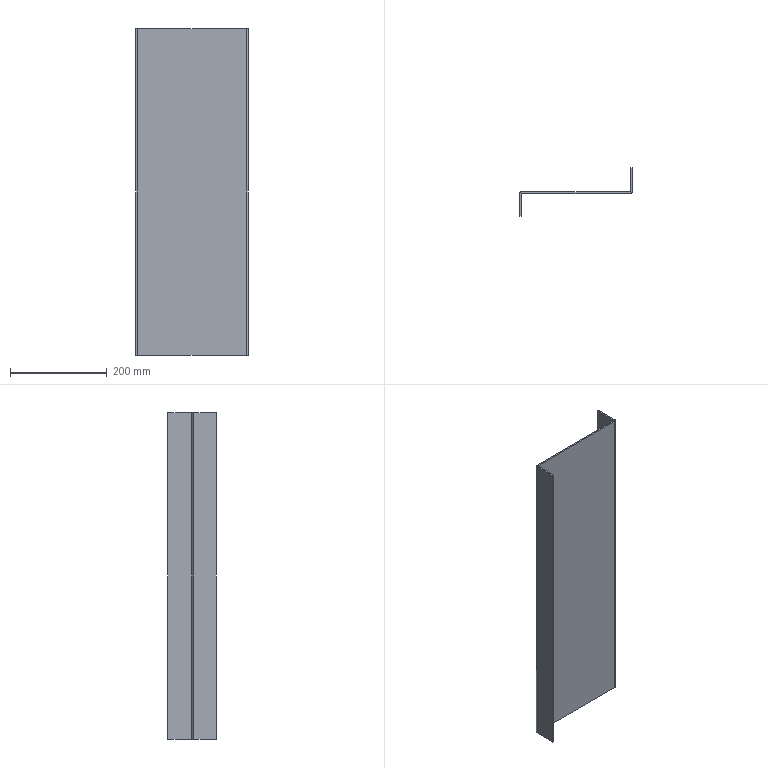Part | STEP file | 中转釜楼梯踏Plate 1 | 1 solid | 14 faces | box 233 x 100 x 674 mm | volume 662921 mm3 | plane 10 | cylinder 4 | commonest cylinder face diameters 2 x2 8 x2
STEP:
#1=CARTESIAN_POINT('',(0.,0.,0.));
#2=DIRECTION('',(0.,0.,1.));
#3=DIRECTION('',(1.,0.,0.));
#4=AXIS2_PLACEMENT_3D('',#1,#2,#3);
#5=CARTESIAN_POINT('',(3.,1.,-337.));
#6=VERTEX_POINT('',#5);
#7=CARTESIAN_POINT('',(3.,50.,-337.));
#8=VERTEX_POINT('',#7);
#9=CARTESIAN_POINT('',(3.,1.,-337.));
#10=DIRECTION('',(0.,1.,0.));
#11=VECTOR('',#10,1.);
#12=LINE('',#9,#11);
#13=CARTESIAN_POINT('',(3.,1.,337.));
#14=DIRECTION('',(-1.,0.,0.));
#15=DIRECTION('',(0.,0.,1.));
#16=AXIS2_PLACEMENT_3D('',#13,#14,#15);
#17=PLANE('',#16);
#18=CARTESIAN_POINT('',(-674.,0.));
#19=DIRECTION('',(0.,1.));
#20=VECTOR('',#19,1.);
#21=LINE('',#18,#20);
#22=(GEOMETRIC_REPRESENTATION_CONTEXT(2)PARAMETRIC_REPRESENTATION_CONTEXT()REPRESENTATION_CONTEXT('',''));
#23=DEFINITIONAL_REPRESENTATION('',(#21),#22);
#24=PCURVE('',#17,#23);
#25=CARTESIAN_POINT('',(-1.,1.,-337.));
#26=DIRECTION('',(0.,0.,1.));
#27=DIRECTION('',(1.,0.,0.));
#28=AXIS2_PLACEMENT_3D('',#25,#26,#27);
#29=PLANE('',#28);
#30=CARTESIAN_POINT('',(4.,0.));
#31=DIRECTION('',(0.,1.));
#32=VECTOR('',#31,1.);
#33=LINE('',#30,#32);
#34=(GEOMETRIC_REPRESENTATION_CONTEXT(2)PARAMETRIC_REPRESENTATION_CONTEXT()REPRESENTATION_CONTEXT('',''));
#35=DEFINITIONAL_REPRESENTATION('',(#33),#34);
#36=PCURVE('',#29,#35);
#37=SURFACE_CURVE('',#12,(#24,#36),.PCURVE_S1.);
#38=EDGE_CURVE('',#6,#8,#37,.T.);
#39=ORIENTED_EDGE('',*,*,#38,.T.);
#40=CARTESIAN_POINT('',(3.,50.,337.));
#41=VERTEX_POINT('',#40);
#42=CARTESIAN_POINT('',(3.,50.,337.));
#43=DIRECTION('',(0.,0.,-1.));
#44=VECTOR('',#43,1.);
#45=LINE('',#42,#44);
#46=CARTESIAN_POINT('',(0.,49.));
#47=DIRECTION('',(-1.,0.));
#48=VECTOR('',#47,1.);
#49=LINE('',#46,#48);
#50=(GEOMETRIC_REPRESENTATION_CONTEXT(2)PARAMETRIC_REPRESENTATION_CONTEXT()REPRESENTATION_CONTEXT('',''));
#51=DEFINITIONAL_REPRESENTATION('',(#49),#50);
#52=PCURVE('',#17,#51);
#53=CARTESIAN_POINT('',(0.,50.,337.));
#54=DIRECTION('',(0.,1.,0.));
#55=DIRECTION('',(0.,0.,1.));
#56=AXIS2_PLACEMENT_3D('',#53,#54,#55);
#57=PLANE('',#56);
#58=CARTESIAN_POINT('',(0.,3.));
#59=DIRECTION('',(-1.,0.));
#60=VECTOR('',#59,1.);
#61=LINE('',#58,#60);
#62=(GEOMETRIC_REPRESENTATION_CONTEXT(2)PARAMETRIC_REPRESENTATION_CONTEXT()REPRESENTATION_CONTEXT('',''));
#63=DEFINITIONAL_REPRESENTATION('',(#61),#62);
#64=PCURVE('',#57,#63);
#65=SURFACE_CURVE('',#45,(#52,#64),.PCURVE_S1.);
#66=EDGE_CURVE('',#41,#8,#65,.T.);
#67=ORIENTED_EDGE('',*,*,#66,.F.);
#68=CARTESIAN_POINT('',(3.,1.,337.));
#69=VERTEX_POINT('',#68);
#70=CARTESIAN_POINT('',(3.,1.,337.));
#71=DIRECTION('',(0.,1.,0.));
#72=VECTOR('',#71,1.);
#73=LINE('',#70,#72);
#74=CARTESIAN_POINT('',(0.,0.));
#75=DIRECTION('',(0.,1.));
#76=VECTOR('',#75,1.);
#77=LINE('',#74,#76);
#78=(GEOMETRIC_REPRESENTATION_CONTEXT(2)PARAMETRIC_REPRESENTATION_CONTEXT()REPRESENTATION_CONTEXT('',''));
#79=DEFINITIONAL_REPRESENTATION('',(#77),#78);
#80=PCURVE('',#17,#79);
#81=CARTESIAN_POINT('',(-1.,1.,337.));
#82=DIRECTION('',(0.,0.,1.));
#83=DIRECTION('',(1.,0.,0.));
#84=AXIS2_PLACEMENT_3D('',#81,#82,#83);
#85=PLANE('',#84);
#86=CARTESIAN_POINT('',(4.,0.));
#87=DIRECTION('',(0.,1.));
#88=VECTOR('',#87,1.);
#89=LINE('',#86,#88);
#90=(GEOMETRIC_REPRESENTATION_CONTEXT(2)PARAMETRIC_REPRESENTATION_CONTEXT()REPRESENTATION_CONTEXT('',''));
#91=DEFINITIONAL_REPRESENTATION('',(#89),#90);
#92=PCURVE('',#85,#91);
#93=SURFACE_CURVE('',#73,(#80,#92),.PCURVE_S1.);
#94=EDGE_CURVE('',#69,#41,#93,.T.);
#95=ORIENTED_EDGE('',*,*,#94,.F.);
#96=CARTESIAN_POINT('',(3.,1.,337.));
#97=DIRECTION('',(0.,0.,-1.));
#98=VECTOR('',#97,1.);
#99=LINE('',#96,#98);
#100=CARTESIAN_POINT('',(0.,0.));
#101=DIRECTION('',(-1.,0.));
#102=VECTOR('',#101,1.);
#103=LINE('',#100,#102);
#104=(GEOMETRIC_REPRESENTATION_CONTEXT(2)PARAMETRIC_REPRESENTATION_CONTEXT()REPRESENTATION_CONTEXT('',''));
#105=DEFINITIONAL_REPRESENTATION('',(#103),#104);
#106=PCURVE('',#17,#105);
#107=CARTESIAN_POINT('',(-1.,1.,337.));
#108=DIRECTION('',(0.,0.,-1.));
#109=DIRECTION('',(-1.,0.,0.));
#110=AXIS2_PLACEMENT_3D('',#107,#108,#109);
#111=CYLINDRICAL_SURFACE('',#110,4.);
#112=CARTESIAN_POINT('',(3.142,0.));
#113=DIRECTION('',(0.,1.));
#114=VECTOR('',#113,1.);
#115=LINE('',#112,#114);
#116=(GEOMETRIC_REPRESENTATION_CONTEXT(2)PARAMETRIC_REPRESENTATION_CONTEXT()REPRESENTATION_CONTEXT('',''));
#117=DEFINITIONAL_REPRESENTATION('',(#115),#116);
#118=PCURVE('',#111,#117);
#119=SURFACE_CURVE('',#99,(#106,#118),.PCURVE_S1.);
#120=EDGE_CURVE('',#69,#6,#119,.T.);
#121=ORIENTED_EDGE('',*,*,#120,.T.);
#122=EDGE_LOOP('',(#39,#67,#95,#121));
#123=FACE_BOUND('',#122,.T.);
#124=ADVANCED_FACE('',(#123),#17,.F.);
#125=CARTESIAN_POINT('',(0.,50.,-337.));
#126=VERTEX_POINT('',#125);
#127=CARTESIAN_POINT('',(0.,50.,-337.));
#128=DIRECTION('',(1.,0.,0.));
#129=VECTOR('',#128,1.);
#130=LINE('',#127,#129);
#131=CARTESIAN_POINT('',(-674.,0.));
#132=DIRECTION('',(0.,1.));
#133=VECTOR('',#132,1.);
#134=LINE('',#131,#133);
#135=(GEOMETRIC_REPRESENTATION_CONTEXT(2)PARAMETRIC_REPRESENTATION_CONTEXT()REPRESENTATION_CONTEXT('',''));
#136=DEFINITIONAL_REPRESENTATION('',(#134),#135);
#137=PCURVE('',#57,#136);
#138=CARTESIAN_POINT('',(1.,49.));
#139=DIRECTION('',(1.,0.));
#140=VECTOR('',#139,1.);
#141=LINE('',#138,#140);
#142=(GEOMETRIC_REPRESENTATION_CONTEXT(2)PARAMETRIC_REPRESENTATION_CONTEXT()REPRESENTATION_CONTEXT('',''));
#143=DEFINITIONAL_REPRESENTATION('',(#141),#142);
#144=PCURVE('',#29,#143);
#145=SURFACE_CURVE('',#130,(#137,#144),.PCURVE_S1.);
#146=EDGE_CURVE('',#126,#8,#145,.T.);
#147=ORIENTED_EDGE('',*,*,#146,.F.);
#148=CARTESIAN_POINT('',(0.,50.,337.));
#149=VERTEX_POINT('',#148);
#150=CARTESIAN_POINT('',(0.,50.,337.));
#151=DIRECTION('',(0.,0.,-1.));
#152=VECTOR('',#151,1.);
#153=LINE('',#150,#152);
#154=CARTESIAN_POINT('',(0.,0.));
#155=DIRECTION('',(-1.,0.));
#156=VECTOR('',#155,1.);
#157=LINE('',#154,#156);
#158=(GEOMETRIC_REPRESENTATION_CONTEXT(2)PARAMETRIC_REPRESENTATION_CONTEXT()REPRESENTATION_CONTEXT('',''));
#159=DEFINITIONAL_REPRESENTATION('',(#157),#158);
#160=PCURVE('',#57,#159);
#161=CARTESIAN_POINT('',(0.,1.,337.));
#162=DIRECTION('',(-1.,0.,0.));
#163=DIRECTION('',(0.,0.,1.));
#164=AXIS2_PLACEMENT_3D('',#161,#162,#163);
#165=PLANE('',#164);
#166=CARTESIAN_POINT('',(0.,49.));
#167=DIRECTION('',(-1.,0.));
#168=VECTOR('',#167,1.);
#169=LINE('',#166,#168);
#170=(GEOMETRIC_REPRESENTATION_CONTEXT(2)PARAMETRIC_REPRESENTATION_CONTEXT()REPRESENTATION_CONTEXT('',''));
#171=DEFINITIONAL_REPRESENTATION('',(#169),#170);
#172=PCURVE('',#165,#171);
#173=SURFACE_CURVE('',#153,(#160,#172),.PCURVE_S1.);
#174=EDGE_CURVE('',#149,#126,#173,.T.);
#175=ORIENTED_EDGE('',*,*,#174,.F.);
#176=CARTESIAN_POINT('',(0.,50.,337.));
#177=DIRECTION('',(1.,0.,0.));
#178=VECTOR('',#177,1.);
#179=LINE('',#176,#178);
#180=CARTESIAN_POINT('',(0.,0.));
#181=DIRECTION('',(0.,1.));
#182=VECTOR('',#181,1.);
#183=LINE('',#180,#182);
#184=(GEOMETRIC_REPRESENTATION_CONTEXT(2)PARAMETRIC_REPRESENTATION_CONTEXT()REPRESENTATION_CONTEXT('',''));
#185=DEFINITIONAL_REPRESENTATION('',(#183),#184);
#186=PCURVE('',#57,#185);
#187=CARTESIAN_POINT('',(1.,49.));
#188=DIRECTION('',(1.,0.));
#189=VECTOR('',#188,1.);
#190=LINE('',#187,#189);
#191=(GEOMETRIC_REPRESENTATION_CONTEXT(2)PARAMETRIC_REPRESENTATION_CONTEXT()REPRESENTATION_CONTEXT('',''));
#192=DEFINITIONAL_REPRESENTATION('',(#190),#191);
#193=PCURVE('',#85,#192);
#194=SURFACE_CURVE('',#179,(#186,#193),.PCURVE_S1.);
#195=EDGE_CURVE('',#149,#41,#194,.T.);
#196=ORIENTED_EDGE('',*,*,#195,.T.);
#197=ORIENTED_EDGE('',*,*,#66,.T.);
#198=EDGE_LOOP('',(#147,#175,#196,#197));
#199=FACE_BOUND('',#198,.T.);
#200=ADVANCED_FACE('',(#199),#57,.T.);
#201=CARTESIAN_POINT('',(0.,1.,-337.));
#202=VERTEX_POINT('',#201);
#203=CARTESIAN_POINT('',(0.,1.,-337.));
#204=DIRECTION('',(0.,1.,0.));
#205=VECTOR('',#204,1.);
#206=LINE('',#203,#205);
#207=CARTESIAN_POINT('',(-674.,0.));
#208=DIRECTION('',(0.,1.));
#209=VECTOR('',#208,1.);
#210=LINE('',#207,#209);
#211=(GEOMETRIC_REPRESENTATION_CONTEXT(2)PARAMETRIC_REPRESENTATION_CONTEXT()REPRESENTATION_CONTEXT('',''));
#212=DEFINITIONAL_REPRESENTATION('',(#210),#211);
#213=PCURVE('',#165,#212);
#214=CARTESIAN_POINT('',(1.,0.));
#215=DIRECTION('',(0.,1.));
#216=VECTOR('',#215,1.);
#217=LINE('',#214,#216);
#218=(GEOMETRIC_REPRESENTATION_CONTEXT(2)PARAMETRIC_REPRESENTATION_CONTEXT()REPRESENTATION_CONTEXT('',''));
#219=DEFINITIONAL_REPRESENTATION('',(#217),#218);
#220=PCURVE('',#29,#219);
#221=SURFACE_CURVE('',#206,(#213,#220),.PCURVE_S1.);
#222=EDGE_CURVE('',#202,#126,#221,.T.);
#223=ORIENTED_EDGE('',*,*,#222,.F.);
#224=CARTESIAN_POINT('',(0.,1.,337.));
#225=VERTEX_POINT('',#224);
#226=CARTESIAN_POINT('',(0.,1.,337.));
#227=DIRECTION('',(0.,0.,-1.));
#228=VECTOR('',#227,1.);
#229=LINE('',#226,#228);
#230=CARTESIAN_POINT('',(0.,0.));
#231=DIRECTION('',(-1.,0.));
#232=VECTOR('',#231,1.);
#233=LINE('',#230,#232);
#234=(GEOMETRIC_REPRESENTATION_CONTEXT(2)PARAMETRIC_REPRESENTATION_CONTEXT()REPRESENTATION_CONTEXT('',''));
#235=DEFINITIONAL_REPRESENTATION('',(#233),#234);
#236=PCURVE('',#165,#235);
#237=CARTESIAN_POINT('',(-1.,1.,337.));
#238=DIRECTION('',(0.,0.,-1.));
#239=DIRECTION('',(-1.,0.,0.));
#240=AXIS2_PLACEMENT_3D('',#237,#238,#239);
#241=CYLINDRICAL_SURFACE('',#240,1.);
#242=CARTESIAN_POINT('',(3.142,0.));
#243=DIRECTION('',(0.,1.));
#244=VECTOR('',#243,1.);
#245=LINE('',#242,#244);
#246=(GEOMETRIC_REPRESENTATION_CONTEXT(2)PARAMETRIC_REPRESENTATION_CONTEXT()REPRESENTATION_CONTEXT('',''));
#247=DEFINITIONAL_REPRESENTATION('',(#245),#246);
#248=PCURVE('',#241,#247);
#249=SURFACE_CURVE('',#229,(#236,#248),.PCURVE_S1.);
#250=EDGE_CURVE('',#225,#202,#249,.T.);
#251=ORIENTED_EDGE('',*,*,#250,.F.);
#252=CARTESIAN_POINT('',(0.,1.,337.));
#253=DIRECTION('',(0.,1.,0.));
#254=VECTOR('',#253,1.);
#255=LINE('',#252,#254);
#256=CARTESIAN_POINT('',(0.,0.));
#257=DIRECTION('',(0.,1.));
#258=VECTOR('',#257,1.);
#259=LINE('',#256,#258);
#260=(GEOMETRIC_REPRESENTATION_CONTEXT(2)PARAMETRIC_REPRESENTATION_CONTEXT()REPRESENTATION_CONTEXT('',''));
#261=DEFINITIONAL_REPRESENTATION('',(#259),#260);
#262=PCURVE('',#165,#261);
#263=CARTESIAN_POINT('',(1.,0.));
#264=DIRECTION('',(0.,1.));
#265=VECTOR('',#264,1.);
#266=LINE('',#263,#265);
#267=(GEOMETRIC_REPRESENTATION_CONTEXT(2)PARAMETRIC_REPRESENTATION_CONTEXT()REPRESENTATION_CONTEXT('',''));
#268=DEFINITIONAL_REPRESENTATION('',(#266),#267);
#269=PCURVE('',#85,#268);
#270=SURFACE_CURVE('',#255,(#262,#269),.PCURVE_S1.);
#271=EDGE_CURVE('',#225,#149,#270,.T.);
#272=ORIENTED_EDGE('',*,*,#271,.T.);
#273=ORIENTED_EDGE('',*,*,#174,.T.);
#274=EDGE_LOOP('',(#223,#251,#272,#273));
#275=FACE_BOUND('',#274,.T.);
#276=ADVANCED_FACE('',(#275),#165,.T.);
#277=ORIENTED_EDGE('',*,*,#250,.F.);
#278=CARTESIAN_POINT('',(-1.,0.,337.));
#279=VERTEX_POINT('',#278);
#280=CARTESIAN_POINT('',(-1.,1.,337.));
#281=DIRECTION('',(0.,0.,1.));
#282=DIRECTION('',(1.,0.,0.));
#283=AXIS2_PLACEMENT_3D('',#280,#281,#282);
#284=CIRCLE('',#283,1.);
#285=CARTESIAN_POINT('',(9.425,0.));
#286=DIRECTION('',(-1.,0.));
#287=VECTOR('',#286,1.);
#288=LINE('',#285,#287);
#289=(GEOMETRIC_REPRESENTATION_CONTEXT(2)PARAMETRIC_REPRESENTATION_CONTEXT()REPRESENTATION_CONTEXT('',''));
#290=DEFINITIONAL_REPRESENTATION('',(#288),#289);
#291=PCURVE('',#241,#290);
#292=CARTESIAN_POINT('',(0.,0.));
#293=DIRECTION('',(1.,0.));
#294=AXIS2_PLACEMENT_2D('',#292,#293);
#295=CIRCLE('',#294,1.);
#296=(GEOMETRIC_REPRESENTATION_CONTEXT(2)PARAMETRIC_REPRESENTATION_CONTEXT()REPRESENTATION_CONTEXT('',''));
#297=DEFINITIONAL_REPRESENTATION('',(#295),#296);
#298=PCURVE('',#85,#297);
#299=SURFACE_CURVE('',#284,(#291,#298),.PCURVE_S1.);
#300=EDGE_CURVE('',#279,#225,#299,.T.);
#301=ORIENTED_EDGE('',*,*,#300,.F.);
#302=CARTESIAN_POINT('',(-1.,0.,-337.));
#303=VERTEX_POINT('',#302);
#304=CARTESIAN_POINT('',(-1.,0.,337.));
#305=DIRECTION('',(0.,0.,-1.));
#306=VECTOR('',#305,1.);
#307=LINE('',#304,#306);
#308=CARTESIAN_POINT('',(4.712,0.));
#309=DIRECTION('',(0.,1.));
#310=VECTOR('',#309,1.);
#311=LINE('',#308,#310);
#312=(GEOMETRIC_REPRESENTATION_CONTEXT(2)PARAMETRIC_REPRESENTATION_CONTEXT()REPRESENTATION_CONTEXT('',''));
#313=DEFINITIONAL_REPRESENTATION('',(#311),#312);
#314=PCURVE('',#241,#313);
#315=CARTESIAN_POINT('',(-226.,0.,337.));
#316=DIRECTION('',(0.,1.,0.));
#317=DIRECTION('',(0.,0.,1.));
#318=AXIS2_PLACEMENT_3D('',#315,#316,#317);
#319=PLANE('',#318);
#320=CARTESIAN_POINT('',(0.,225.));
#321=DIRECTION('',(-1.,0.));
#322=VECTOR('',#321,1.);
#323=LINE('',#320,#322);
#324=(GEOMETRIC_REPRESENTATION_CONTEXT(2)PARAMETRIC_REPRESENTATION_CONTEXT()REPRESENTATION_CONTEXT('',''));
#325=DEFINITIONAL_REPRESENTATION('',(#323),#324);
#326=PCURVE('',#319,#325);
#327=SURFACE_CURVE('',#307,(#314,#326),.PCURVE_S1.);
#328=EDGE_CURVE('',#279,#303,#327,.T.);
#329=ORIENTED_EDGE('',*,*,#328,.T.);
#330=CARTESIAN_POINT('',(-1.,1.,-337.));
#331=DIRECTION('',(0.,0.,1.));
#332=DIRECTION('',(1.,0.,0.));
#333=AXIS2_PLACEMENT_3D('',#330,#331,#332);
#334=CIRCLE('',#333,1.);
#335=CARTESIAN_POINT('',(9.425,674.));
#336=DIRECTION('',(-1.,0.));
#337=VECTOR('',#336,1.);
#338=LINE('',#335,#337);
#339=(GEOMETRIC_REPRESENTATION_CONTEXT(2)PARAMETRIC_REPRESENTATION_CONTEXT()REPRESENTATION_CONTEXT('',''));
#340=DEFINITIONAL_REPRESENTATION('',(#338),#339);
#341=PCURVE('',#241,#340);
#342=CARTESIAN_POINT('',(0.,0.));
#343=DIRECTION('',(1.,0.));
#344=AXIS2_PLACEMENT_2D('',#342,#343);
#345=CIRCLE('',#344,1.);
#346=(GEOMETRIC_REPRESENTATION_CONTEXT(2)PARAMETRIC_REPRESENTATION_CONTEXT()REPRESENTATION_CONTEXT('',''));
#347=DEFINITIONAL_REPRESENTATION('',(#345),#346);
#348=PCURVE('',#29,#347);
#349=SURFACE_CURVE('',#334,(#341,#348),.PCURVE_S1.);
#350=EDGE_CURVE('',#303,#202,#349,.T.);
#351=ORIENTED_EDGE('',*,*,#350,.T.);
#352=EDGE_LOOP('',(#277,#301,#329,#351));
#353=FACE_BOUND('',#352,.F.);
#354=ADVANCED_FACE('',(#353),#241,.F.);
#355=CARTESIAN_POINT('',(-226.,0.,-337.));
#356=VERTEX_POINT('',#355);
#357=CARTESIAN_POINT('',(-226.,0.,-337.));
#358=DIRECTION('',(1.,0.,0.));
#359=VECTOR('',#358,1.);
#360=LINE('',#357,#359);
#361=CARTESIAN_POINT('',(-674.,0.));
#362=DIRECTION('',(0.,1.));
#363=VECTOR('',#362,1.);
#364=LINE('',#361,#363);
#365=(GEOMETRIC_REPRESENTATION_CONTEXT(2)PARAMETRIC_REPRESENTATION_CONTEXT()REPRESENTATION_CONTEXT('',''));
#366=DEFINITIONAL_REPRESENTATION('',(#364),#365);
#367=PCURVE('',#319,#366);
#368=CARTESIAN_POINT('',(-225.,-1.));
#369=DIRECTION('',(1.,0.));
#370=VECTOR('',#369,1.);
#371=LINE('',#368,#370);
#372=(GEOMETRIC_REPRESENTATION_CONTEXT(2)PARAMETRIC_REPRESENTATION_CONTEXT()REPRESENTATION_CONTEXT('',''));
#373=DEFINITIONAL_REPRESENTATION('',(#371),#372);
#374=PCURVE('',#29,#373);
#375=SURFACE_CURVE('',#360,(#367,#374),.PCURVE_S1.);
#376=EDGE_CURVE('',#356,#303,#375,.T.);
#377=ORIENTED_EDGE('',*,*,#376,.F.);
#378=CARTESIAN_POINT('',(-226.,0.,337.));
#379=VERTEX_POINT('',#378);
#380=CARTESIAN_POINT('',(-226.,0.,337.));
#381=DIRECTION('',(0.,0.,-1.));
#382=VECTOR('',#381,1.);
#383=LINE('',#380,#382);
#384=CARTESIAN_POINT('',(0.,0.));
#385=DIRECTION('',(-1.,0.));
#386=VECTOR('',#385,1.);
#387=LINE('',#384,#386);
#388=(GEOMETRIC_REPRESENTATION_CONTEXT(2)PARAMETRIC_REPRESENTATION_CONTEXT()REPRESENTATION_CONTEXT('',''));
#389=DEFINITIONAL_REPRESENTATION('',(#387),#388);
#390=PCURVE('',#319,#389);
#391=CARTESIAN_POINT('',(-226.,-4.,337.));
#392=DIRECTION('',(0.,0.,-1.));
#393=DIRECTION('',(-1.,0.,0.));
#394=AXIS2_PLACEMENT_3D('',#391,#392,#393);
#395=CYLINDRICAL_SURFACE('',#394,4.);
#396=CARTESIAN_POINT('',(1.571,0.));
#397=DIRECTION('',(0.,1.));
#398=VECTOR('',#397,1.);
#399=LINE('',#396,#398);
#400=(GEOMETRIC_REPRESENTATION_CONTEXT(2)PARAMETRIC_REPRESENTATION_CONTEXT()REPRESENTATION_CONTEXT('',''));
#401=DEFINITIONAL_REPRESENTATION('',(#399),#400);
#402=PCURVE('',#395,#401);
#403=SURFACE_CURVE('',#383,(#390,#402),.PCURVE_S1.);
#404=EDGE_CURVE('',#379,#356,#403,.T.);
#405=ORIENTED_EDGE('',*,*,#404,.F.);
#406=CARTESIAN_POINT('',(-226.,0.,337.));
#407=DIRECTION('',(1.,0.,0.));
#408=VECTOR('',#407,1.);
#409=LINE('',#406,#408);
#410=CARTESIAN_POINT('',(0.,0.));
#411=DIRECTION('',(0.,1.));
#412=VECTOR('',#411,1.);
#413=LINE('',#410,#412);
#414=(GEOMETRIC_REPRESENTATION_CONTEXT(2)PARAMETRIC_REPRESENTATION_CONTEXT()REPRESENTATION_CONTEXT('',''));
#415=DEFINITIONAL_REPRESENTATION('',(#413),#414);
#416=PCURVE('',#319,#415);
#417=CARTESIAN_POINT('',(-225.,-1.));
#418=DIRECTION('',(1.,0.));
#419=VECTOR('',#418,1.);
#420=LINE('',#417,#419);
#421=(GEOMETRIC_REPRESENTATION_CONTEXT(2)PARAMETRIC_REPRESENTATION_CONTEXT()REPRESENTATION_CONTEXT('',''));
#422=DEFINITIONAL_REPRESENTATION('',(#420),#421);
#423=PCURVE('',#85,#422);
#424=SURFACE_CURVE('',#409,(#416,#423),.PCURVE_S1.);
#425=EDGE_CURVE('',#379,#279,#424,.T.);
#426=ORIENTED_EDGE('',*,*,#425,.T.);
#427=ORIENTED_EDGE('',*,*,#328,.T.);
#428=EDGE_LOOP('',(#377,#405,#426,#427));
#429=FACE_BOUND('',#428,.T.);
#430=ADVANCED_FACE('',(#429),#319,.T.);
#431=CARTESIAN_POINT('',(-230.,-4.,-337.));
#432=VERTEX_POINT('',#431);
#433=CARTESIAN_POINT('',(-226.,-4.,-337.));
#434=DIRECTION('',(0.,0.,-1.));
#435=DIRECTION('',(1.,0.,0.));
#436=AXIS2_PLACEMENT_3D('',#433,#434,#435);
#437=CIRCLE('',#436,4.);
#438=CARTESIAN_POINT('',(-3.142,674.));
#439=DIRECTION('',(1.,0.));
#440=VECTOR('',#439,1.);
#441=LINE('',#438,#440);
#442=(GEOMETRIC_REPRESENTATION_CONTEXT(2)PARAMETRIC_REPRESENTATION_CONTEXT()REPRESENTATION_CONTEXT('',''));
#443=DEFINITIONAL_REPRESENTATION('',(#441),#442);
#444=PCURVE('',#395,#443);
#445=CARTESIAN_POINT('',(-221.,-5.));
#446=CARTESIAN_POINT('',(-221.,-11.928));
#447=CARTESIAN_POINT('',(-227.,-8.464));
#448=CARTESIAN_POINT('',(-233.,-5.));
#449=CARTESIAN_POINT('',(-227.,-1.536));
#450=CARTESIAN_POINT('',(-221.,1.928));
#451=CARTESIAN_POINT('',(-221.,-5.));
#452=(BOUNDED_CURVE()B_SPLINE_CURVE(2,(#445,#446,#447,#448,#449,#450,#451),.UNSPECIFIED.,.T.,.F.)B_SPLINE_CURVE_WITH_KNOTS((1,2,2,2,2,1),(-2.094,0.,2.094,4.189,6.283,8.378),.UNSPECIFIED.)CURVE()GEOMETRIC_REPRESENTATION_ITEM()RATIONAL_B_SPLINE_CURVE((1.,0.5,1.,0.5,1.,0.5,1.))REPRESENTATION_ITEM(''));
#453=(GEOMETRIC_REPRESENTATION_CONTEXT(2)PARAMETRIC_REPRESENTATION_CONTEXT()REPRESENTATION_CONTEXT('',''));
#454=DEFINITIONAL_REPRESENTATION('',(#452),#453);
#455=PCURVE('',#29,#454);
#456=SURFACE_CURVE('',#437,(#444,#455),.PCURVE_S1.);
#457=EDGE_CURVE('',#432,#356,#456,.T.);
#458=ORIENTED_EDGE('',*,*,#457,.F.);
#459=CARTESIAN_POINT('',(-230.,-4.,337.));
#460=VERTEX_POINT('',#459);
#461=CARTESIAN_POINT('',(-230.,-4.,337.));
#462=DIRECTION('',(0.,0.,-1.));
#463=VECTOR('',#462,1.);
#464=LINE('',#461,#463);
#465=CARTESIAN_POINT('',(0.,0.));
#466=DIRECTION('',(0.,1.));
#467=VECTOR('',#466,1.);
#468=LINE('',#465,#467);
#469=(GEOMETRIC_REPRESENTATION_CONTEXT(2)PARAMETRIC_REPRESENTATION_CONTEXT()REPRESENTATION_CONTEXT('',''));
#470=DEFINITIONAL_REPRESENTATION('',(#468),#469);
#471=PCURVE('',#395,#470);
#472=CARTESIAN_POINT('',(-230.,-4.,337.));
#473=DIRECTION('',(-1.,0.,0.));
#474=DIRECTION('',(0.,0.,1.));
#475=AXIS2_PLACEMENT_3D('',#472,#473,#474);
#476=PLANE('',#475);
#477=CARTESIAN_POINT('',(0.,0.));
#478=DIRECTION('',(-1.,0.));
#479=VECTOR('',#478,1.);
#480=LINE('',#477,#479);
#481=(GEOMETRIC_REPRESENTATION_CONTEXT(2)PARAMETRIC_REPRESENTATION_CONTEXT()REPRESENTATION_CONTEXT('',''));
#482=DEFINITIONAL_REPRESENTATION('',(#480),#481);
#483=PCURVE('',#476,#482);
#484=SURFACE_CURVE('',#464,(#471,#483),.PCURVE_S1.);
#485=EDGE_CURVE('',#460,#432,#484,.T.);
#486=ORIENTED_EDGE('',*,*,#485,.F.);
#487=CARTESIAN_POINT('',(-226.,-4.,337.));
#488=DIRECTION('',(0.,0.,-1.));
#489=DIRECTION('',(1.,0.,0.));
#490=AXIS2_PLACEMENT_3D('',#487,#488,#489);
#491=CIRCLE('',#490,4.);
#492=CARTESIAN_POINT('',(-3.142,0.));
#493=DIRECTION('',(1.,0.));
#494=VECTOR('',#493,1.);
#495=LINE('',#492,#494);
#496=(GEOMETRIC_REPRESENTATION_CONTEXT(2)PARAMETRIC_REPRESENTATION_CONTEXT()REPRESENTATION_CONTEXT('',''));
#497=DEFINITIONAL_REPRESENTATION('',(#495),#496);
#498=PCURVE('',#395,#497);
#499=CARTESIAN_POINT('',(-221.,-5.));
#500=CARTESIAN_POINT('',(-221.,-11.928));
#501=CARTESIAN_POINT('',(-227.,-8.464));
#502=CARTESIAN_POINT('',(-233.,-5.));
#503=CARTESIAN_POINT('',(-227.,-1.536));
#504=CARTESIAN_POINT('',(-221.,1.928));
#505=CARTESIAN_POINT('',(-221.,-5.));
#506=(BOUNDED_CURVE()B_SPLINE_CURVE(2,(#499,#500,#501,#502,#503,#504,#505),.UNSPECIFIED.,.T.,.F.)B_SPLINE_CURVE_WITH_KNOTS((1,2,2,2,2,1),(-2.094,0.,2.094,4.189,6.283,8.378),.UNSPECIFIED.)CURVE()GEOMETRIC_REPRESENTATION_ITEM()RATIONAL_B_SPLINE_CURVE((1.,0.5,1.,0.5,1.,0.5,1.))REPRESENTATION_ITEM(''));
#507=(GEOMETRIC_REPRESENTATION_CONTEXT(2)PARAMETRIC_REPRESENTATION_CONTEXT()REPRESENTATION_CONTEXT('',''));
#508=DEFINITIONAL_REPRESENTATION('',(#506),#507);
#509=PCURVE('',#85,#508);
#510=SURFACE_CURVE('',#491,(#498,#509),.PCURVE_S1.);
#511=EDGE_CURVE('',#460,#379,#510,.T.);
#512=ORIENTED_EDGE('',*,*,#511,.T.);
#513=ORIENTED_EDGE('',*,*,#404,.T.);
#514=EDGE_LOOP('',(#458,#486,#512,#513));
#515=FACE_BOUND('',#514,.T.);
#516=ADVANCED_FACE('',(#515),#395,.T.);
#517=CARTESIAN_POINT('',(-230.,-50.,-337.));
#518=VERTEX_POINT('',#517);
#519=CARTESIAN_POINT('',(-230.,-4.,-337.));
#520=DIRECTION('',(0.,1.,0.));
#521=VECTOR('',#520,1.);
#522=LINE('',#519,#521);
#523=CARTESIAN_POINT('',(-674.,0.));
#524=DIRECTION('',(0.,1.));
#525=VECTOR('',#524,1.);
#526=LINE('',#523,#525);
#527=(GEOMETRIC_REPRESENTATION_CONTEXT(2)PARAMETRIC_REPRESENTATION_CONTEXT()REPRESENTATION_CONTEXT('',''));
#528=DEFINITIONAL_REPRESENTATION('',(#526),#527);
#529=PCURVE('',#476,#528);
#530=CARTESIAN_POINT('',(-229.,-5.));
#531=DIRECTION('',(0.,1.));
#532=VECTOR('',#531,1.);
#533=LINE('',#530,#532);
#534=(GEOMETRIC_REPRESENTATION_CONTEXT(2)PARAMETRIC_REPRESENTATION_CONTEXT()REPRESENTATION_CONTEXT('',''));
#535=DEFINITIONAL_REPRESENTATION('',(#533),#534);
#536=PCURVE('',#29,#535);
#537=SURFACE_CURVE('',#522,(#529,#536),.PCURVE_S1.);
#538=EDGE_CURVE('',#518,#432,#537,.T.);
#539=ORIENTED_EDGE('',*,*,#538,.F.);
#540=CARTESIAN_POINT('',(-230.,-50.,337.));
#541=VERTEX_POINT('',#540);
#542=CARTESIAN_POINT('',(-230.,-50.,337.));
#543=DIRECTION('',(0.,0.,-1.));
#544=VECTOR('',#543,1.);
#545=LINE('',#542,#544);
#546=CARTESIAN_POINT('',(0.,-46.));
#547=DIRECTION('',(-1.,0.));
#548=VECTOR('',#547,1.);
#549=LINE('',#546,#548);
#550=(GEOMETRIC_REPRESENTATION_CONTEXT(2)PARAMETRIC_REPRESENTATION_CONTEXT()REPRESENTATION_CONTEXT('',''));
#551=DEFINITIONAL_REPRESENTATION('',(#549),#550);
#552=PCURVE('',#476,#551);
#553=CARTESIAN_POINT('',(-227.,-50.,337.));
#554=DIRECTION('',(0.,-1.,0.));
#555=DIRECTION('',(0.,0.,-1.));
#556=AXIS2_PLACEMENT_3D('',#553,#554,#555);
#557=PLANE('',#556);
#558=CARTESIAN_POINT('',(0.,-3.));
#559=DIRECTION('',(1.,0.));
#560=VECTOR('',#559,1.);
#561=LINE('',#558,#560);
#562=(GEOMETRIC_REPRESENTATION_CONTEXT(2)PARAMETRIC_REPRESENTATION_CONTEXT()REPRESENTATION_CONTEXT('',''));
#563=DEFINITIONAL_REPRESENTATION('',(#561),#562);
#564=PCURVE('',#557,#563);
#565=SURFACE_CURVE('',#545,(#552,#564),.PCURVE_S1.);
#566=EDGE_CURVE('',#541,#518,#565,.T.);
#567=ORIENTED_EDGE('',*,*,#566,.F.);
#568=CARTESIAN_POINT('',(-230.,-4.,337.));
#569=DIRECTION('',(0.,1.,0.));
#570=VECTOR('',#569,1.);
#571=LINE('',#568,#570);
#572=CARTESIAN_POINT('',(0.,0.));
#573=DIRECTION('',(0.,1.));
#574=VECTOR('',#573,1.);
#575=LINE('',#572,#574);
#576=(GEOMETRIC_REPRESENTATION_CONTEXT(2)PARAMETRIC_REPRESENTATION_CONTEXT()REPRESENTATION_CONTEXT('',''));
#577=DEFINITIONAL_REPRESENTATION('',(#575),#576);
#578=PCURVE('',#476,#577);
#579=CARTESIAN_POINT('',(-229.,-5.));
#580=DIRECTION('',(0.,1.));
#581=VECTOR('',#580,1.);
#582=LINE('',#579,#581);
#583=(GEOMETRIC_REPRESENTATION_CONTEXT(2)PARAMETRIC_REPRESENTATION_CONTEXT()REPRESENTATION_CONTEXT('',''));
#584=DEFINITIONAL_REPRESENTATION('',(#582),#583);
#585=PCURVE('',#85,#584);
#586=SURFACE_CURVE('',#571,(#578,#585),.PCURVE_S1.);
#587=EDGE_CURVE('',#541,#460,#586,.T.);
#588=ORIENTED_EDGE('',*,*,#587,.T.);
#589=ORIENTED_EDGE('',*,*,#485,.T.);
#590=EDGE_LOOP('',(#539,#567,#588,#589));
#591=FACE_BOUND('',#590,.T.);
#592=ADVANCED_FACE('',(#591),#476,.T.);
#593=CARTESIAN_POINT('',(-227.,-50.,-337.));
#594=VERTEX_POINT('',#593);
#595=CARTESIAN_POINT('',(-227.,-50.,-337.));
#596=DIRECTION('',(-1.,0.,0.));
#597=VECTOR('',#596,1.);
#598=LINE('',#595,#597);
#599=CARTESIAN_POINT('',(674.,0.));
#600=DIRECTION('',(0.,-1.));
#601=VECTOR('',#600,1.);
#602=LINE('',#599,#601);
#603=(GEOMETRIC_REPRESENTATION_CONTEXT(2)PARAMETRIC_REPRESENTATION_CONTEXT()REPRESENTATION_CONTEXT('',''));
#604=DEFINITIONAL_REPRESENTATION('',(#602),#603);
#605=PCURVE('',#557,#604);
#606=CARTESIAN_POINT('',(-226.,-51.));
#607=DIRECTION('',(-1.,0.));
#608=VECTOR('',#607,1.);
#609=LINE('',#606,#608);
#610=(GEOMETRIC_REPRESENTATION_CONTEXT(2)PARAMETRIC_REPRESENTATION_CONTEXT()REPRESENTATION_CONTEXT('',''));
#611=DEFINITIONAL_REPRESENTATION('',(#609),#610);
#612=PCURVE('',#29,#611);
#613=SURFACE_CURVE('',#598,(#605,#612),.PCURVE_S1.);
#614=EDGE_CURVE('',#594,#518,#613,.T.);
#615=ORIENTED_EDGE('',*,*,#614,.F.);
#616=CARTESIAN_POINT('',(-227.,-50.,337.));
#617=VERTEX_POINT('',#616);
#618=CARTESIAN_POINT('',(-227.,-50.,337.));
#619=DIRECTION('',(0.,0.,-1.));
#620=VECTOR('',#619,1.);
#621=LINE('',#618,#620);
#622=CARTESIAN_POINT('',(0.,0.));
#623=DIRECTION('',(1.,0.));
#624=VECTOR('',#623,1.);
#625=LINE('',#622,#624);
#626=(GEOMETRIC_REPRESENTATION_CONTEXT(2)PARAMETRIC_REPRESENTATION_CONTEXT()REPRESENTATION_CONTEXT('',''));
#627=DEFINITIONAL_REPRESENTATION('',(#625),#626);
#628=PCURVE('',#557,#627);
#629=CARTESIAN_POINT('',(-227.,-4.,337.));
#630=DIRECTION('',(-1.,0.,0.));
#631=DIRECTION('',(0.,0.,1.));
#632=AXIS2_PLACEMENT_3D('',#629,#630,#631);
#633=PLANE('',#632);
#634=CARTESIAN_POINT('',(0.,-46.));
#635=DIRECTION('',(-1.,0.));
#636=VECTOR('',#635,1.);
#637=LINE('',#634,#636);
#638=(GEOMETRIC_REPRESENTATION_CONTEXT(2)PARAMETRIC_REPRESENTATION_CONTEXT()REPRESENTATION_CONTEXT('',''));
#639=DEFINITIONAL_REPRESENTATION('',(#637),#638);
#640=PCURVE('',#633,#639);
#641=SURFACE_CURVE('',#621,(#628,#640),.PCURVE_S1.);
#642=EDGE_CURVE('',#617,#594,#641,.T.);
#643=ORIENTED_EDGE('',*,*,#642,.F.);
#644=CARTESIAN_POINT('',(-227.,-50.,337.));
#645=DIRECTION('',(-1.,0.,0.));
#646=VECTOR('',#645,1.);
#647=LINE('',#644,#646);
#648=CARTESIAN_POINT('',(0.,0.));
#649=DIRECTION('',(0.,-1.));
#650=VECTOR('',#649,1.);
#651=LINE('',#648,#650);
#652=(GEOMETRIC_REPRESENTATION_CONTEXT(2)PARAMETRIC_REPRESENTATION_CONTEXT()REPRESENTATION_CONTEXT('',''));
#653=DEFINITIONAL_REPRESENTATION('',(#651),#652);
#654=PCURVE('',#557,#653);
#655=CARTESIAN_POINT('',(-226.,-51.));
#656=DIRECTION('',(-1.,0.));
#657=VECTOR('',#656,1.);
#658=LINE('',#655,#657);
#659=(GEOMETRIC_REPRESENTATION_CONTEXT(2)PARAMETRIC_REPRESENTATION_CONTEXT()REPRESENTATION_CONTEXT('',''));
#660=DEFINITIONAL_REPRESENTATION('',(#658),#659);
#661=PCURVE('',#85,#660);
#662=SURFACE_CURVE('',#647,(#654,#661),.PCURVE_S1.);
#663=EDGE_CURVE('',#617,#541,#662,.T.);
#664=ORIENTED_EDGE('',*,*,#663,.T.);
#665=ORIENTED_EDGE('',*,*,#566,.T.);
#666=EDGE_LOOP('',(#615,#643,#664,#665));
#667=FACE_BOUND('',#666,.T.);
#668=ADVANCED_FACE('',(#667),#557,.T.);
#669=CARTESIAN_POINT('',(-227.,-4.,-337.));
#670=VERTEX_POINT('',#669);
#671=CARTESIAN_POINT('',(-227.,-4.,-337.));
#672=DIRECTION('',(0.,1.,0.));
#673=VECTOR('',#672,1.);
#674=LINE('',#671,#673);
#675=CARTESIAN_POINT('',(-674.,0.));
#676=DIRECTION('',(0.,1.));
#677=VECTOR('',#676,1.);
#678=LINE('',#675,#677);
#679=(GEOMETRIC_REPRESENTATION_CONTEXT(2)PARAMETRIC_REPRESENTATION_CONTEXT()REPRESENTATION_CONTEXT('',''));
#680=DEFINITIONAL_REPRESENTATION('',(#678),#679);
#681=PCURVE('',#633,#680);
#682=CARTESIAN_POINT('',(-226.,-5.));
#683=DIRECTION('',(0.,1.));
#684=VECTOR('',#683,1.);
#685=LINE('',#682,#684);
#686=(GEOMETRIC_REPRESENTATION_CONTEXT(2)PARAMETRIC_REPRESENTATION_CONTEXT()REPRESENTATION_CONTEXT('',''));
#687=DEFINITIONAL_REPRESENTATION('',(#685),#686);
#688=PCURVE('',#29,#687);
#689=SURFACE_CURVE('',#674,(#681,#688),.PCURVE_S1.);
#690=EDGE_CURVE('',#594,#670,#689,.T.);
#691=ORIENTED_EDGE('',*,*,#690,.T.);
#692=CARTESIAN_POINT('',(-227.,-4.,337.));
#693=VERTEX_POINT('',#692);
#694=CARTESIAN_POINT('',(-227.,-4.,337.));
#695=DIRECTION('',(0.,0.,-1.));
#696=VECTOR('',#695,1.);
#697=LINE('',#694,#696);
#698=CARTESIAN_POINT('',(0.,0.));
#699=DIRECTION('',(-1.,0.));
#700=VECTOR('',#699,1.);
#701=LINE('',#698,#700);
#702=(GEOMETRIC_REPRESENTATION_CONTEXT(2)PARAMETRIC_REPRESENTATION_CONTEXT()REPRESENTATION_CONTEXT('',''));
#703=DEFINITIONAL_REPRESENTATION('',(#701),#702);
#704=PCURVE('',#633,#703);
#705=CARTESIAN_POINT('',(-226.,-4.,337.));
#706=DIRECTION('',(0.,0.,-1.));
#707=DIRECTION('',(-1.,0.,0.));
#708=AXIS2_PLACEMENT_3D('',#705,#706,#707);
#709=CYLINDRICAL_SURFACE('',#708,1.);
#710=CARTESIAN_POINT('',(0.,0.));
#711=DIRECTION('',(0.,1.));
#712=VECTOR('',#711,1.);
#713=LINE('',#710,#712);
#714=(GEOMETRIC_REPRESENTATION_CONTEXT(2)PARAMETRIC_REPRESENTATION_CONTEXT()REPRESENTATION_CONTEXT('',''));
#715=DEFINITIONAL_REPRESENTATION('',(#713),#714);
#716=PCURVE('',#709,#715);
#717=SURFACE_CURVE('',#697,(#704,#716),.PCURVE_S1.);
#718=EDGE_CURVE('',#693,#670,#717,.T.);
#719=ORIENTED_EDGE('',*,*,#718,.F.);
#720=CARTESIAN_POINT('',(-227.,-4.,337.));
#721=DIRECTION('',(0.,1.,0.));
#722=VECTOR('',#721,1.);
#723=LINE('',#720,#722);
#724=CARTESIAN_POINT('',(0.,0.));
#725=DIRECTION('',(0.,1.));
#726=VECTOR('',#725,1.);
#727=LINE('',#724,#726);
#728=(GEOMETRIC_REPRESENTATION_CONTEXT(2)PARAMETRIC_REPRESENTATION_CONTEXT()REPRESENTATION_CONTEXT('',''));
#729=DEFINITIONAL_REPRESENTATION('',(#727),#728);
#730=PCURVE('',#633,#729);
#731=CARTESIAN_POINT('',(-226.,-5.));
#732=DIRECTION('',(0.,1.));
#733=VECTOR('',#732,1.);
#734=LINE('',#731,#733);
#735=(GEOMETRIC_REPRESENTATION_CONTEXT(2)PARAMETRIC_REPRESENTATION_CONTEXT()REPRESENTATION_CONTEXT('',''));
#736=DEFINITIONAL_REPRESENTATION('',(#734),#735);
#737=PCURVE('',#85,#736);
#738=SURFACE_CURVE('',#723,(#730,#737),.PCURVE_S1.);
#739=EDGE_CURVE('',#617,#693,#738,.T.);
#740=ORIENTED_EDGE('',*,*,#739,.F.);
#741=ORIENTED_EDGE('',*,*,#642,.T.);
#742=EDGE_LOOP('',(#691,#719,#740,#741));
#743=FACE_BOUND('',#742,.T.);
#744=ADVANCED_FACE('',(#743),#633,.F.);
#745=ORIENTED_EDGE('',*,*,#718,.F.);
#746=CARTESIAN_POINT('',(-226.,-3.,337.));
#747=VERTEX_POINT('',#746);
#748=CARTESIAN_POINT('',(-226.,-4.,337.));
#749=DIRECTION('',(0.,0.,-1.));
#750=DIRECTION('',(1.,0.,0.));
#751=AXIS2_PLACEMENT_3D('',#748,#749,#750);
#752=CIRCLE('',#751,1.);
#753=CARTESIAN_POINT('',(-3.142,0.));
#754=DIRECTION('',(1.,0.));
#755=VECTOR('',#754,1.);
#756=LINE('',#753,#755);
#757=(GEOMETRIC_REPRESENTATION_CONTEXT(2)PARAMETRIC_REPRESENTATION_CONTEXT()REPRESENTATION_CONTEXT('',''));
#758=DEFINITIONAL_REPRESENTATION('',(#756),#757);
#759=PCURVE('',#709,#758);
#760=CARTESIAN_POINT('',(-224.,-5.));
#761=CARTESIAN_POINT('',(-224.,-6.732));
#762=CARTESIAN_POINT('',(-225.5,-5.866));
#763=CARTESIAN_POINT('',(-227.,-5.));
#764=CARTESIAN_POINT('',(-225.5,-4.134));
#765=CARTESIAN_POINT('',(-224.,-3.268));
#766=CARTESIAN_POINT('',(-224.,-5.));
#767=(BOUNDED_CURVE()B_SPLINE_CURVE(2,(#760,#761,#762,#763,#764,#765,#766),.UNSPECIFIED.,.T.,.F.)B_SPLINE_CURVE_WITH_KNOTS((1,2,2,2,2,1),(-2.094,0.,2.094,4.189,6.283,8.378),.UNSPECIFIED.)CURVE()GEOMETRIC_REPRESENTATION_ITEM()RATIONAL_B_SPLINE_CURVE((1.,0.5,1.,0.5,1.,0.5,1.))REPRESENTATION_ITEM(''));
#768=(GEOMETRIC_REPRESENTATION_CONTEXT(2)PARAMETRIC_REPRESENTATION_CONTEXT()REPRESENTATION_CONTEXT('',''));
#769=DEFINITIONAL_REPRESENTATION('',(#767),#768);
#770=PCURVE('',#85,#769);
#771=SURFACE_CURVE('',#752,(#759,#770),.PCURVE_S1.);
#772=EDGE_CURVE('',#693,#747,#771,.T.);
#773=ORIENTED_EDGE('',*,*,#772,.T.);
#774=CARTESIAN_POINT('',(-226.,-3.,-337.));
#775=VERTEX_POINT('',#774);
#776=CARTESIAN_POINT('',(-226.,-3.,337.));
#777=DIRECTION('',(0.,0.,-1.));
#778=VECTOR('',#777,1.);
#779=LINE('',#776,#778);
#780=CARTESIAN_POINT('',(1.571,0.));
#781=DIRECTION('',(0.,1.));
#782=VECTOR('',#781,1.);
#783=LINE('',#780,#782);
#784=(GEOMETRIC_REPRESENTATION_CONTEXT(2)PARAMETRIC_REPRESENTATION_CONTEXT()REPRESENTATION_CONTEXT('',''));
#785=DEFINITIONAL_REPRESENTATION('',(#783),#784);
#786=PCURVE('',#709,#785);
#787=CARTESIAN_POINT('',(-226.,-3.,337.));
#788=DIRECTION('',(0.,1.,0.));
#789=DIRECTION('',(0.,0.,1.));
#790=AXIS2_PLACEMENT_3D('',#787,#788,#789);
#791=PLANE('',#790);
#792=CARTESIAN_POINT('',(0.,0.));
#793=DIRECTION('',(-1.,0.));
#794=VECTOR('',#793,1.);
#795=LINE('',#792,#794);
#796=(GEOMETRIC_REPRESENTATION_CONTEXT(2)PARAMETRIC_REPRESENTATION_CONTEXT()REPRESENTATION_CONTEXT('',''));
#797=DEFINITIONAL_REPRESENTATION('',(#795),#796);
#798=PCURVE('',#791,#797);
#799=SURFACE_CURVE('',#779,(#786,#798),.PCURVE_S1.);
#800=EDGE_CURVE('',#747,#775,#799,.T.);
#801=ORIENTED_EDGE('',*,*,#800,.T.);
#802=CARTESIAN_POINT('',(-226.,-4.,-337.));
#803=DIRECTION('',(0.,0.,-1.));
#804=DIRECTION('',(1.,0.,0.));
#805=AXIS2_PLACEMENT_3D('',#802,#803,#804);
#806=CIRCLE('',#805,1.);
#807=CARTESIAN_POINT('',(-3.142,674.));
#808=DIRECTION('',(1.,0.));
#809=VECTOR('',#808,1.);
#810=LINE('',#807,#809);
#811=(GEOMETRIC_REPRESENTATION_CONTEXT(2)PARAMETRIC_REPRESENTATION_CONTEXT()REPRESENTATION_CONTEXT('',''));
#812=DEFINITIONAL_REPRESENTATION('',(#810),#811);
#813=PCURVE('',#709,#812);
#814=CARTESIAN_POINT('',(-224.,-5.));
#815=CARTESIAN_POINT('',(-224.,-6.732));
#816=CARTESIAN_POINT('',(-225.5,-5.866));
#817=CARTESIAN_POINT('',(-227.,-5.));
#818=CARTESIAN_POINT('',(-225.5,-4.134));
#819=CARTESIAN_POINT('',(-224.,-3.268));
#820=CARTESIAN_POINT('',(-224.,-5.));
#821=(BOUNDED_CURVE()B_SPLINE_CURVE(2,(#814,#815,#816,#817,#818,#819,#820),.UNSPECIFIED.,.T.,.F.)B_SPLINE_CURVE_WITH_KNOTS((1,2,2,2,2,1),(-2.094,0.,2.094,4.189,6.283,8.378),.UNSPECIFIED.)CURVE()GEOMETRIC_REPRESENTATION_ITEM()RATIONAL_B_SPLINE_CURVE((1.,0.5,1.,0.5,1.,0.5,1.))REPRESENTATION_ITEM(''));
#822=(GEOMETRIC_REPRESENTATION_CONTEXT(2)PARAMETRIC_REPRESENTATION_CONTEXT()REPRESENTATION_CONTEXT('',''));
#823=DEFINITIONAL_REPRESENTATION('',(#821),#822);
#824=PCURVE('',#29,#823);
#825=SURFACE_CURVE('',#806,(#813,#824),.PCURVE_S1.);
#826=EDGE_CURVE('',#670,#775,#825,.T.);
#827=ORIENTED_EDGE('',*,*,#826,.F.);
#828=EDGE_LOOP('',(#745,#773,#801,#827));
#829=FACE_BOUND('',#828,.F.);
#830=ADVANCED_FACE('',(#829),#709,.F.);
#831=CARTESIAN_POINT('',(-1.,-3.,-337.));
#832=VERTEX_POINT('',#831);
#833=CARTESIAN_POINT('',(-226.,-3.,-337.));
#834=DIRECTION('',(1.,0.,0.));
#835=VECTOR('',#834,1.);
#836=LINE('',#833,#835);
#837=CARTESIAN_POINT('',(-674.,0.));
#838=DIRECTION('',(0.,1.));
#839=VECTOR('',#838,1.);
#840=LINE('',#837,#839);
#841=(GEOMETRIC_REPRESENTATION_CONTEXT(2)PARAMETRIC_REPRESENTATION_CONTEXT()REPRESENTATION_CONTEXT('',''));
#842=DEFINITIONAL_REPRESENTATION('',(#840),#841);
#843=PCURVE('',#791,#842);
#844=CARTESIAN_POINT('',(-225.,-4.));
#845=DIRECTION('',(1.,0.));
#846=VECTOR('',#845,1.);
#847=LINE('',#844,#846);
#848=(GEOMETRIC_REPRESENTATION_CONTEXT(2)PARAMETRIC_REPRESENTATION_CONTEXT()REPRESENTATION_CONTEXT('',''));
#849=DEFINITIONAL_REPRESENTATION('',(#847),#848);
#850=PCURVE('',#29,#849);
#851=SURFACE_CURVE('',#836,(#843,#850),.PCURVE_S1.);
#852=EDGE_CURVE('',#775,#832,#851,.T.);
#853=ORIENTED_EDGE('',*,*,#852,.T.);
#854=CARTESIAN_POINT('',(-1.,-3.,337.));
#855=VERTEX_POINT('',#854);
#856=CARTESIAN_POINT('',(-1.,-3.,337.));
#857=DIRECTION('',(0.,0.,-1.));
#858=VECTOR('',#857,1.);
#859=LINE('',#856,#858);
#860=CARTESIAN_POINT('',(0.,225.));
#861=DIRECTION('',(-1.,0.));
#862=VECTOR('',#861,1.);
#863=LINE('',#860,#862);
#864=(GEOMETRIC_REPRESENTATION_CONTEXT(2)PARAMETRIC_REPRESENTATION_CONTEXT()REPRESENTATION_CONTEXT('',''));
#865=DEFINITIONAL_REPRESENTATION('',(#863),#864);
#866=PCURVE('',#791,#865);
#867=CARTESIAN_POINT('',(4.712,0.));
#868=DIRECTION('',(0.,1.));
#869=VECTOR('',#868,1.);
#870=LINE('',#867,#869);
#871=(GEOMETRIC_REPRESENTATION_CONTEXT(2)PARAMETRIC_REPRESENTATION_CONTEXT()REPRESENTATION_CONTEXT('',''));
#872=DEFINITIONAL_REPRESENTATION('',(#870),#871);
#873=PCURVE('',#111,#872);
#874=SURFACE_CURVE('',#859,(#866,#873),.PCURVE_S1.);
#875=EDGE_CURVE('',#855,#832,#874,.T.);
#876=ORIENTED_EDGE('',*,*,#875,.F.);
#877=CARTESIAN_POINT('',(-226.,-3.,337.));
#878=DIRECTION('',(1.,0.,0.));
#879=VECTOR('',#878,1.);
#880=LINE('',#877,#879);
#881=CARTESIAN_POINT('',(0.,0.));
#882=DIRECTION('',(0.,1.));
#883=VECTOR('',#882,1.);
#884=LINE('',#881,#883);
#885=(GEOMETRIC_REPRESENTATION_CONTEXT(2)PARAMETRIC_REPRESENTATION_CONTEXT()REPRESENTATION_CONTEXT('',''));
#886=DEFINITIONAL_REPRESENTATION('',(#884),#885);
#887=PCURVE('',#791,#886);
#888=CARTESIAN_POINT('',(-225.,-4.));
#889=DIRECTION('',(1.,0.));
#890=VECTOR('',#889,1.);
#891=LINE('',#888,#890);
#892=(GEOMETRIC_REPRESENTATION_CONTEXT(2)PARAMETRIC_REPRESENTATION_CONTEXT()REPRESENTATION_CONTEXT('',''));
#893=DEFINITIONAL_REPRESENTATION('',(#891),#892);
#894=PCURVE('',#85,#893);
#895=SURFACE_CURVE('',#880,(#887,#894),.PCURVE_S1.);
#896=EDGE_CURVE('',#747,#855,#895,.T.);
#897=ORIENTED_EDGE('',*,*,#896,.F.);
#898=ORIENTED_EDGE('',*,*,#800,.T.);
#899=EDGE_LOOP('',(#853,#876,#897,#898));
#900=FACE_BOUND('',#899,.T.);
#901=ADVANCED_FACE('',(#900),#791,.F.);
#902=CARTESIAN_POINT('',(-1.,1.,-337.));
#903=DIRECTION('',(0.,0.,1.));
#904=DIRECTION('',(1.,0.,0.));
#905=AXIS2_PLACEMENT_3D('',#902,#903,#904);
#906=CIRCLE('',#905,4.);
#907=CARTESIAN_POINT('',(9.425,674.));
#908=DIRECTION('',(-1.,0.));
#909=VECTOR('',#908,1.);
#910=LINE('',#907,#909);
#911=(GEOMETRIC_REPRESENTATION_CONTEXT(2)PARAMETRIC_REPRESENTATION_CONTEXT()REPRESENTATION_CONTEXT('',''));
#912=DEFINITIONAL_REPRESENTATION('',(#910),#911);
#913=PCURVE('',#111,#912);
#914=CARTESIAN_POINT('',(0.,0.));
#915=DIRECTION('',(1.,0.));
#916=AXIS2_PLACEMENT_2D('',#914,#915);
#917=CIRCLE('',#916,4.);
#918=(GEOMETRIC_REPRESENTATION_CONTEXT(2)PARAMETRIC_REPRESENTATION_CONTEXT()REPRESENTATION_CONTEXT('',''));
#919=DEFINITIONAL_REPRESENTATION('',(#917),#918);
#920=PCURVE('',#29,#919);
#921=SURFACE_CURVE('',#906,(#913,#920),.PCURVE_S1.);
#922=EDGE_CURVE('',#832,#6,#921,.T.);
#923=ORIENTED_EDGE('',*,*,#922,.T.);
#924=ORIENTED_EDGE('',*,*,#120,.F.);
#925=CARTESIAN_POINT('',(-1.,1.,337.));
#926=DIRECTION('',(0.,0.,1.));
#927=DIRECTION('',(1.,0.,0.));
#928=AXIS2_PLACEMENT_3D('',#925,#926,#927);
#929=CIRCLE('',#928,4.);
#930=CARTESIAN_POINT('',(9.425,0.));
#931=DIRECTION('',(-1.,0.));
#932=VECTOR('',#931,1.);
#933=LINE('',#930,#932);
#934=(GEOMETRIC_REPRESENTATION_CONTEXT(2)PARAMETRIC_REPRESENTATION_CONTEXT()REPRESENTATION_CONTEXT('',''));
#935=DEFINITIONAL_REPRESENTATION('',(#933),#934);
#936=PCURVE('',#111,#935);
#937=CARTESIAN_POINT('',(0.,0.));
#938=DIRECTION('',(1.,0.));
#939=AXIS2_PLACEMENT_2D('',#937,#938);
#940=CIRCLE('',#939,4.);
#941=(GEOMETRIC_REPRESENTATION_CONTEXT(2)PARAMETRIC_REPRESENTATION_CONTEXT()REPRESENTATION_CONTEXT('',''));
#942=DEFINITIONAL_REPRESENTATION('',(#940),#941);
#943=PCURVE('',#85,#942);
#944=SURFACE_CURVE('',#929,(#936,#943),.PCURVE_S1.);
#945=EDGE_CURVE('',#855,#69,#944,.T.);
#946=ORIENTED_EDGE('',*,*,#945,.F.);
#947=ORIENTED_EDGE('',*,*,#875,.T.);
#948=EDGE_LOOP('',(#923,#924,#946,#947));
#949=FACE_BOUND('',#948,.T.);
#950=ADVANCED_FACE('',(#949),#111,.T.);
#951=ORIENTED_EDGE('',*,*,#94,.T.);
#952=ORIENTED_EDGE('',*,*,#195,.F.);
#953=ORIENTED_EDGE('',*,*,#271,.F.);
#954=ORIENTED_EDGE('',*,*,#300,.F.);
#955=ORIENTED_EDGE('',*,*,#425,.F.);
#956=ORIENTED_EDGE('',*,*,#511,.F.);
#957=ORIENTED_EDGE('',*,*,#587,.F.);
#958=ORIENTED_EDGE('',*,*,#663,.F.);
#959=ORIENTED_EDGE('',*,*,#739,.T.);
#960=ORIENTED_EDGE('',*,*,#772,.T.);
#961=ORIENTED_EDGE('',*,*,#896,.T.);
#962=ORIENTED_EDGE('',*,*,#945,.T.);
#963=EDGE_LOOP('',(#951,#952,#953,#954,#955,#956,#957,#958,#959,#960,#961,#962));
#964=FACE_BOUND('',#963,.T.);
#965=ADVANCED_FACE('',(#964),#85,.T.);
#966=ORIENTED_EDGE('',*,*,#38,.F.);
#967=ORIENTED_EDGE('',*,*,#922,.F.);
#968=ORIENTED_EDGE('',*,*,#852,.F.);
#969=ORIENTED_EDGE('',*,*,#826,.F.);
#970=ORIENTED_EDGE('',*,*,#690,.F.);
#971=ORIENTED_EDGE('',*,*,#614,.T.);
#972=ORIENTED_EDGE('',*,*,#538,.T.);
#973=ORIENTED_EDGE('',*,*,#457,.T.);
#974=ORIENTED_EDGE('',*,*,#376,.T.);
#975=ORIENTED_EDGE('',*,*,#350,.T.);
#976=ORIENTED_EDGE('',*,*,#222,.T.);
#977=ORIENTED_EDGE('',*,*,#146,.T.);
#978=EDGE_LOOP('',(#966,#967,#968,#969,#970,#971,#972,#973,#974,#975,#976,#977));
#979=FACE_BOUND('',#978,.T.);
#980=ADVANCED_FACE('',(#979),#29,.F.);
#981=CLOSED_SHELL('',(#124,#200,#276,#354,#430,#516,#592,#668,#744,#830,#901,#950,#965,#980));
#982=MANIFOLD_SOLID_BREP('',#981);
#983=(LENGTH_UNIT()NAMED_UNIT(*)SI_UNIT(.MILLI.,.METRE.));
#984=UNCERTAINTY_MEASURE_WITH_UNIT(LENGTH_MEASURE(0.0000001),#983,'','');
#985=(NAMED_UNIT(*)PLANE_ANGLE_UNIT()SI_UNIT($,.RADIAN.));
#986=(NAMED_UNIT(*)SI_UNIT($,.STERADIAN.)SOLID_ANGLE_UNIT());
#987=(GEOMETRIC_REPRESENTATION_CONTEXT(3)GLOBAL_UNCERTAINTY_ASSIGNED_CONTEXT((#984))GLOBAL_UNIT_ASSIGNED_CONTEXT((#983,#985,#986))REPRESENTATION_CONTEXT('',''));
#988=ADVANCED_BREP_SHAPE_REPRESENTATION('',(#4,#982),#987);